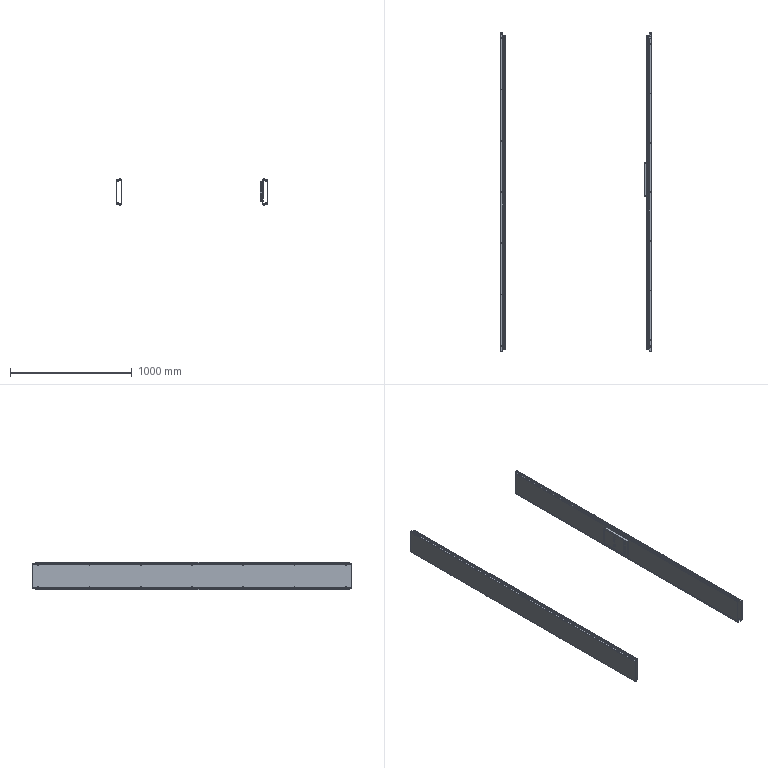Part | 37 solids | 1353 faces | box 1240 x 2616 x 227 mm | volume 5629616 mm3 | plane 836 | cylinder 407 | spline 110 | commonest cylinder face diameters 6 x56 6.2 x56 8 x56 12 x56 6.4 x48 0.6 x40